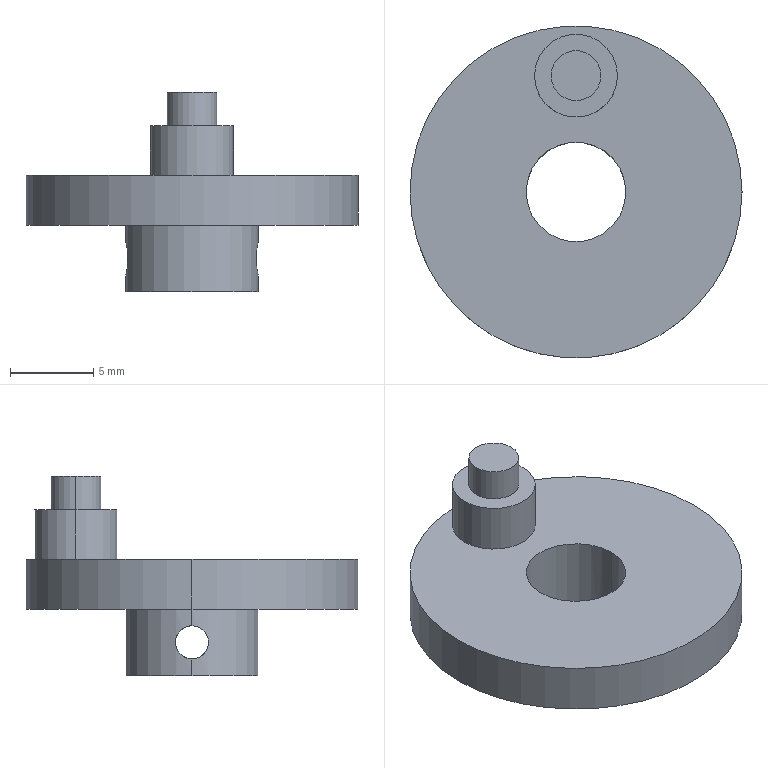Part | SolidWorks | features ICE 5, Extrusion 1 | 1 solid | 19 faces | box 20 x 20 x 12 mm | volume 1012 mm3 | cylinder 14 | plane 5 | commonest cylinder face diameters 2 x4 3 x2 5 x2 6 x2 8 x2 20 x2
STEP:
#1=CARTESIAN_POINT('',(3.,0.,-1.));
#2=VERTEX_POINT('',#1);
#3=CARTESIAN_POINT('',(3.,0.,-3.));
#4=VERTEX_POINT('',#3);
#5=CARTESIAN_POINT('',(3.,0.,-1.));
#6=CARTESIAN_POINT('',(3.,-0.1312,-1.));
#7=CARTESIAN_POINT('',(2.991,-0.2636,-1.027));
#8=CARTESIAN_POINT('',(2.96,-0.5049,-1.127));
#9=CARTESIAN_POINT('',(2.938,-0.6149,-1.201));
#10=CARTESIAN_POINT('',(2.893,-0.7996,-1.385));
#11=CARTESIAN_POINT('',(2.871,-0.8728,-1.494));
#12=CARTESIAN_POINT('',(2.838,-0.9739,-1.737));
#13=CARTESIAN_POINT('',(2.828,-1.,-1.868));
#14=CARTESIAN_POINT('',(2.828,-1.,-2.132));
#15=CARTESIAN_POINT('',(2.838,-0.9733,-2.264));
#16=CARTESIAN_POINT('',(2.871,-0.8731,-2.505));
#17=CARTESIAN_POINT('',(2.893,-0.7989,-2.615));
#18=CARTESIAN_POINT('',(2.938,-0.6156,-2.799));
#19=CARTESIAN_POINT('',(2.96,-0.5055,-2.873));
#20=CARTESIAN_POINT('',(2.991,-0.2638,-2.973));
#21=CARTESIAN_POINT('',(3.,-0.1331,-3.));
#22=CARTESIAN_POINT('',(3.,0.,-3.));
#23=B_SPLINE_CURVE_WITH_KNOTS('',3,(#5,#6,#7,#8,#9,#10,#11,#12,#13,#14,#15,#16,#17,#18,#19,#20,#21,#22),.UNSPECIFIED.,.F.,.F.,(4,2,2,2,2,2,2,2,4),(0.003149,0.003543,0.003936,0.00433,0.004723,0.005117,0.00551,0.005904,0.006298),.UNSPECIFIED.);
#24=EDGE_CURVE('',#2,#4,#23,.T.);
#25=ORIENTED_EDGE('',*,*,#24,.F.);
#26=CARTESIAN_POINT('',(4.,0.,-1.));
#27=VERTEX_POINT('',#26);
#28=CARTESIAN_POINT('',(-5.,0.,-1.));
#29=DIRECTION('',(1.,0.,0.));
#30=VECTOR('',#29,1000.);
#31=LINE('',#28,#30);
#32=EDGE_CURVE('',#2,#27,#31,.T.);
#33=ORIENTED_EDGE('',*,*,#32,.T.);
#34=CARTESIAN_POINT('',(4.,0.,-3.));
#35=VERTEX_POINT('',#34);
#36=CARTESIAN_POINT('',(4.,0.,-3.));
#37=CARTESIAN_POINT('',(4.,-0.1327,-3.));
#38=CARTESIAN_POINT('',(3.993,-0.2629,-2.974));
#39=CARTESIAN_POINT('',(3.97,-0.5049,-2.873));
#40=CARTESIAN_POINT('',(3.953,-0.6155,-2.799));
#41=CARTESIAN_POINT('',(3.92,-0.7991,-2.615));
#42=CARTESIAN_POINT('',(3.904,-0.8735,-2.504));
#43=CARTESIAN_POINT('',(3.88,-0.9734,-2.263));
#44=CARTESIAN_POINT('',(3.873,-0.9999,-2.131));
#45=CARTESIAN_POINT('',(3.873,-1.,-1.869));
#46=CARTESIAN_POINT('',(3.88,-0.974,-1.738));
#47=CARTESIAN_POINT('',(3.904,-0.8732,-1.495));
#48=CARTESIAN_POINT('',(3.92,-0.7996,-1.385));
#49=CARTESIAN_POINT('',(3.954,-0.6143,-1.2));
#50=CARTESIAN_POINT('',(3.97,-0.5041,-1.127));
#51=CARTESIAN_POINT('',(3.993,-0.2626,-1.026));
#52=CARTESIAN_POINT('',(4.,-0.1308,-1.));
#53=CARTESIAN_POINT('',(4.,0.,-1.));
#54=B_SPLINE_CURVE_WITH_KNOTS('',3,(#36,#37,#38,#39,#40,#41,#42,#43,#44,#45,#46,#47,#48,#49,#50,#51,#52,#53),.UNSPECIFIED.,.F.,.F.,(4,2,2,2,2,2,2,2,4),(0.,0.0003924,0.0007847,0.001177,0.001569,0.001962,0.002354,0.002747,0.003139),.UNSPECIFIED.);
#55=EDGE_CURVE('',#35,#27,#54,.T.);
#56=ORIENTED_EDGE('',*,*,#55,.F.);
#57=CARTESIAN_POINT('',(-5.,0.,-3.));
#58=DIRECTION('',(1.,0.,0.));
#59=VECTOR('',#58,1000.);
#60=LINE('',#57,#59);
#61=EDGE_CURVE('',#4,#35,#60,.T.);
#62=ORIENTED_EDGE('',*,*,#61,.F.);
#63=EDGE_LOOP('',(#25,#33,#56,#62));
#64=FACE_OUTER_BOUND('',#63,.T.);
#65=CARTESIAN_POINT('',(-5.,0.,-2.));
#66=DIRECTION('',(1.,0.,0.));
#67=DIRECTION('',(0.,0.,-1.));
#68=AXIS2_PLACEMENT_3D('',#65,#66,#67);
#69=CYLINDRICAL_SURFACE('',#68,1.);
#70=ADVANCED_FACE('',(#64),#69,.F.);
#71=CARTESIAN_POINT('',(-4.,0.,-1.));
#72=VERTEX_POINT('',#71);
#73=CARTESIAN_POINT('',(-4.,0.,-3.));
#74=VERTEX_POINT('',#73);
#75=CARTESIAN_POINT('',(-4.,0.,-1.));
#76=CARTESIAN_POINT('',(-4.,-0.1308,-1.));
#77=CARTESIAN_POINT('',(-3.993,-0.2629,-1.026));
#78=CARTESIAN_POINT('',(-3.97,-0.5038,-1.126));
#79=CARTESIAN_POINT('',(-3.954,-0.6146,-1.2));
#80=CARTESIAN_POINT('',(-3.92,-0.7991,-1.385));
#81=CARTESIAN_POINT('',(-3.904,-0.8727,-1.494));
#82=CARTESIAN_POINT('',(-3.88,-0.9739,-1.738));
#83=CARTESIAN_POINT('',(-3.873,-1.,-1.868));
#84=CARTESIAN_POINT('',(-3.873,-1.,-2.132));
#85=CARTESIAN_POINT('',(-3.88,-0.9737,-2.263));
#86=CARTESIAN_POINT('',(-3.904,-0.8736,-2.504));
#87=CARTESIAN_POINT('',(-3.92,-0.7992,-2.615));
#88=CARTESIAN_POINT('',(-3.953,-0.6158,-2.799));
#89=CARTESIAN_POINT('',(-3.97,-0.5048,-2.873));
#90=CARTESIAN_POINT('',(-3.993,-0.2641,-2.973));
#91=CARTESIAN_POINT('',(-4.,-0.1327,-3.));
#92=CARTESIAN_POINT('',(-4.,0.,-3.));
#93=B_SPLINE_CURVE_WITH_KNOTS('',3,(#75,#76,#77,#78,#79,#80,#81,#82,#83,#84,#85,#86,#87,#88,#89,#90,#91,#92),.UNSPECIFIED.,.F.,.F.,(4,2,2,2,2,2,2,2,4),(0.003139,0.003531,0.003923,0.004316,0.004708,0.0051,0.005493,0.005885,0.006277),.UNSPECIFIED.);
#94=EDGE_CURVE('',#72,#74,#93,.T.);
#95=ORIENTED_EDGE('',*,*,#94,.F.);
#96=CARTESIAN_POINT('',(-3.,0.,-1.));
#97=VERTEX_POINT('',#96);
#98=CARTESIAN_POINT('',(-5.,0.,-1.));
#99=DIRECTION('',(1.,0.,0.));
#100=VECTOR('',#99,1000.);
#101=LINE('',#98,#100);
#102=EDGE_CURVE('',#72,#97,#101,.T.);
#103=ORIENTED_EDGE('',*,*,#102,.T.);
#104=CARTESIAN_POINT('',(-3.,0.,-3.));
#105=VERTEX_POINT('',#104);
#106=CARTESIAN_POINT('',(-3.,0.,-3.));
#107=CARTESIAN_POINT('',(-3.,-0.1312,-3.));
#108=CARTESIAN_POINT('',(-2.991,-0.2636,-2.973));
#109=CARTESIAN_POINT('',(-2.96,-0.5049,-2.873));
#110=CARTESIAN_POINT('',(-2.938,-0.6149,-2.799));
#111=CARTESIAN_POINT('',(-2.893,-0.7996,-2.615));
#112=CARTESIAN_POINT('',(-2.871,-0.8728,-2.506));
#113=CARTESIAN_POINT('',(-2.838,-0.9739,-2.263));
#114=CARTESIAN_POINT('',(-2.828,-1.,-2.132));
#115=CARTESIAN_POINT('',(-2.828,-1.,-1.868));
#116=CARTESIAN_POINT('',(-2.838,-0.9733,-1.736));
#117=CARTESIAN_POINT('',(-2.871,-0.8731,-1.495));
#118=CARTESIAN_POINT('',(-2.893,-0.7989,-1.385));
#119=CARTESIAN_POINT('',(-2.938,-0.6156,-1.201));
#120=CARTESIAN_POINT('',(-2.96,-0.5055,-1.127));
#121=CARTESIAN_POINT('',(-2.991,-0.2638,-1.027));
#122=CARTESIAN_POINT('',(-3.,-0.1331,-1.));
#123=CARTESIAN_POINT('',(-3.,0.,-1.));
#124=B_SPLINE_CURVE_WITH_KNOTS('',3,(#106,#107,#108,#109,#110,#111,#112,#113,#114,#115,#116,#117,#118,#119,#120,#121,#122,#123),.UNSPECIFIED.,.F.,.F.,(4,2,2,2,2,2,2,2,4),(0.003149,0.003543,0.003936,0.00433,0.004723,0.005117,0.00551,0.005904,0.006298),.UNSPECIFIED.);
#125=EDGE_CURVE('',#105,#97,#124,.T.);
#126=ORIENTED_EDGE('',*,*,#125,.F.);
#127=CARTESIAN_POINT('',(-5.,0.,-3.));
#128=DIRECTION('',(1.,0.,0.));
#129=VECTOR('',#128,1000.);
#130=LINE('',#127,#129);
#131=EDGE_CURVE('',#74,#105,#130,.T.);
#132=ORIENTED_EDGE('',*,*,#131,.F.);
#133=EDGE_LOOP('',(#95,#103,#126,#132));
#134=FACE_OUTER_BOUND('',#133,.T.);
#135=CARTESIAN_POINT('',(-5.,0.,-2.));
#136=DIRECTION('',(1.,0.,0.));
#137=DIRECTION('',(0.,0.,-1.));
#138=AXIS2_PLACEMENT_3D('',#135,#136,#137);
#139=CYLINDRICAL_SURFACE('',#138,1.);
#140=ADVANCED_FACE('',(#134),#139,.F.);
#141=CARTESIAN_POINT('',(-4.,0.,-4.));
#142=VERTEX_POINT('',#141);
#143=CARTESIAN_POINT('',(4.,0.,-4.));
#144=VERTEX_POINT('',#143);
#145=CARTESIAN_POINT('',(0.,0.,-4.));
#146=DIRECTION('',(0.,0.,-1.));
#147=DIRECTION('',(-1.,0.,0.));
#148=AXIS2_PLACEMENT_3D('',#145,#146,#147);
#149=CIRCLE('',#148,4.);
#150=EDGE_CURVE('',#142,#144,#149,.T.);
#151=ORIENTED_EDGE('',*,*,#150,.F.);
#152=CARTESIAN_POINT('',(-4.,0.,-4.));
#153=DIRECTION('',(0.,0.,1.));
#154=VECTOR('',#153,1000.);
#155=LINE('',#152,#154);
#156=EDGE_CURVE('',#142,#74,#155,.T.);
#157=ORIENTED_EDGE('',*,*,#156,.T.);
#158=CARTESIAN_POINT('',(-4.,0.,-3.));
#159=CARTESIAN_POINT('',(-4.,0.1327,-3.));
#160=CARTESIAN_POINT('',(-3.993,0.2629,-2.974));
#161=CARTESIAN_POINT('',(-3.97,0.5049,-2.873));
#162=CARTESIAN_POINT('',(-3.953,0.6155,-2.799));
#163=CARTESIAN_POINT('',(-3.92,0.7991,-2.615));
#164=CARTESIAN_POINT('',(-3.904,0.8735,-2.504));
#165=CARTESIAN_POINT('',(-3.88,0.9734,-2.263));
#166=CARTESIAN_POINT('',(-3.873,0.9999,-2.131));
#167=CARTESIAN_POINT('',(-3.873,1.,-1.869));
#168=CARTESIAN_POINT('',(-3.88,0.974,-1.738));
#169=CARTESIAN_POINT('',(-3.904,0.8732,-1.495));
#170=CARTESIAN_POINT('',(-3.92,0.7996,-1.385));
#171=CARTESIAN_POINT('',(-3.954,0.6143,-1.2));
#172=CARTESIAN_POINT('',(-3.97,0.5041,-1.127));
#173=CARTESIAN_POINT('',(-3.993,0.2626,-1.026));
#174=CARTESIAN_POINT('',(-4.,0.1308,-1.));
#175=CARTESIAN_POINT('',(-4.,0.,-1.));
#176=B_SPLINE_CURVE_WITH_KNOTS('',3,(#158,#159,#160,#161,#162,#163,#164,#165,#166,#167,#168,#169,#170,#171,#172,#173,#174,#175),.UNSPECIFIED.,.F.,.F.,(4,2,2,2,2,2,2,2,4),(0.,0.0003924,0.0007847,0.001177,0.001569,0.001962,0.002354,0.002747,0.003139),.UNSPECIFIED.);
#177=EDGE_CURVE('',#74,#72,#176,.T.);
#178=ORIENTED_EDGE('',*,*,#177,.T.);
#179=CARTESIAN_POINT('',(-4.,0.,0.));
#180=VERTEX_POINT('',#179);
#181=CARTESIAN_POINT('',(-4.,0.,-4.));
#182=DIRECTION('',(0.,0.,1.));
#183=VECTOR('',#182,1000.);
#184=LINE('',#181,#183);
#185=EDGE_CURVE('',#72,#180,#184,.T.);
#186=ORIENTED_EDGE('',*,*,#185,.T.);
#187=CARTESIAN_POINT('',(4.,0.,0.));
#188=VERTEX_POINT('',#187);
#189=CARTESIAN_POINT('',(0.,0.,0.));
#190=DIRECTION('',(0.,0.,-1.));
#191=DIRECTION('',(1.,0.,0.));
#192=AXIS2_PLACEMENT_3D('',#189,#190,#191);
#193=CIRCLE('',#192,4.);
#194=EDGE_CURVE('',#180,#188,#193,.T.);
#195=ORIENTED_EDGE('',*,*,#194,.T.);
#196=CARTESIAN_POINT('',(4.,0.,-4.));
#197=DIRECTION('',(0.,0.,1.));
#198=VECTOR('',#197,1000.);
#199=LINE('',#196,#198);
#200=EDGE_CURVE('',#27,#188,#199,.T.);
#201=ORIENTED_EDGE('',*,*,#200,.F.);
#202=CARTESIAN_POINT('',(4.,0.,-1.));
#203=CARTESIAN_POINT('',(4.,0.1308,-1.));
#204=CARTESIAN_POINT('',(3.993,0.2629,-1.026));
#205=CARTESIAN_POINT('',(3.97,0.5038,-1.126));
#206=CARTESIAN_POINT('',(3.954,0.6146,-1.2));
#207=CARTESIAN_POINT('',(3.92,0.7991,-1.385));
#208=CARTESIAN_POINT('',(3.904,0.8727,-1.494));
#209=CARTESIAN_POINT('',(3.88,0.9739,-1.738));
#210=CARTESIAN_POINT('',(3.873,1.,-1.868));
#211=CARTESIAN_POINT('',(3.873,1.,-2.132));
#212=CARTESIAN_POINT('',(3.88,0.9737,-2.263));
#213=CARTESIAN_POINT('',(3.904,0.8736,-2.504));
#214=CARTESIAN_POINT('',(3.92,0.7992,-2.615));
#215=CARTESIAN_POINT('',(3.953,0.6158,-2.799));
#216=CARTESIAN_POINT('',(3.97,0.5048,-2.873));
#217=CARTESIAN_POINT('',(3.993,0.2641,-2.973));
#218=CARTESIAN_POINT('',(4.,0.1327,-3.));
#219=CARTESIAN_POINT('',(4.,0.,-3.));
#220=B_SPLINE_CURVE_WITH_KNOTS('',3,(#202,#203,#204,#205,#206,#207,#208,#209,#210,#211,#212,#213,#214,#215,#216,#217,#218,#219),.UNSPECIFIED.,.F.,.F.,(4,2,2,2,2,2,2,2,4),(0.003139,0.003531,0.003923,0.004316,0.004708,0.0051,0.005493,0.005885,0.006277),.UNSPECIFIED.);
#221=EDGE_CURVE('',#27,#35,#220,.T.);
#222=ORIENTED_EDGE('',*,*,#221,.T.);
#223=CARTESIAN_POINT('',(4.,0.,-4.));
#224=DIRECTION('',(0.,0.,1.));
#225=VECTOR('',#224,1000.);
#226=LINE('',#223,#225);
#227=EDGE_CURVE('',#144,#35,#226,.T.);
#228=ORIENTED_EDGE('',*,*,#227,.F.);
#229=EDGE_LOOP('',(#151,#157,#178,#186,#195,#201,#222,#228));
#230=FACE_OUTER_BOUND('',#229,.T.);
#231=CARTESIAN_POINT('',(0.,0.,-4.));
#232=DIRECTION('',(0.,0.,1.));
#233=DIRECTION('',(1.,0.,0.));
#234=AXIS2_PLACEMENT_3D('',#231,#232,#233);
#235=CYLINDRICAL_SURFACE('',#234,4.);
#236=ADVANCED_FACE('',(#230),#235,.T.);
#237=CARTESIAN_POINT('',(-3.,0.,3.));
#238=VERTEX_POINT('',#237);
#239=CARTESIAN_POINT('',(3.,0.,3.));
#240=VERTEX_POINT('',#239);
#241=CARTESIAN_POINT('',(0.,0.,3.));
#242=DIRECTION('',(0.,0.,1.));
#243=DIRECTION('',(1.,0.,0.));
#244=AXIS2_PLACEMENT_3D('',#241,#242,#243);
#245=CIRCLE('',#244,3.);
#246=EDGE_CURVE('',#238,#240,#245,.T.);
#247=ORIENTED_EDGE('',*,*,#246,.T.);
#248=CARTESIAN_POINT('',(3.,0.,24.));
#249=DIRECTION('',(0.,0.,-1.));
#250=VECTOR('',#249,1000.);
#251=LINE('',#248,#250);
#252=EDGE_CURVE('',#240,#2,#251,.T.);
#253=ORIENTED_EDGE('',*,*,#252,.T.);
#254=ORIENTED_EDGE('',*,*,#24,.T.);
#255=CARTESIAN_POINT('',(3.,0.,-4.));
#256=VERTEX_POINT('',#255);
#257=CARTESIAN_POINT('',(3.,0.,24.));
#258=DIRECTION('',(0.,0.,-1.));
#259=VECTOR('',#258,1000.);
#260=LINE('',#257,#259);
#261=EDGE_CURVE('',#4,#256,#260,.T.);
#262=ORIENTED_EDGE('',*,*,#261,.T.);
#263=CARTESIAN_POINT('',(-3.,0.,-4.));
#264=VERTEX_POINT('',#263);
#265=CARTESIAN_POINT('',(0.,0.,-4.));
#266=DIRECTION('',(0.,0.,-1.));
#267=DIRECTION('',(-1.,0.,0.));
#268=AXIS2_PLACEMENT_3D('',#265,#266,#267);
#269=CIRCLE('',#268,3.);
#270=EDGE_CURVE('',#256,#264,#269,.T.);
#271=ORIENTED_EDGE('',*,*,#270,.T.);
#272=CARTESIAN_POINT('',(-3.,0.,24.));
#273=DIRECTION('',(0.,0.,-1.));
#274=VECTOR('',#273,1000.);
#275=LINE('',#272,#274);
#276=EDGE_CURVE('',#105,#264,#275,.T.);
#277=ORIENTED_EDGE('',*,*,#276,.F.);
#278=ORIENTED_EDGE('',*,*,#125,.T.);
#279=CARTESIAN_POINT('',(-3.,0.,24.));
#280=DIRECTION('',(0.,0.,-1.));
#281=VECTOR('',#280,1000.);
#282=LINE('',#279,#281);
#283=EDGE_CURVE('',#238,#97,#282,.T.);
#284=ORIENTED_EDGE('',*,*,#283,.F.);
#285=EDGE_LOOP('',(#247,#253,#254,#262,#271,#277,#278,#284));
#286=FACE_OUTER_BOUND('',#285,.T.);
#287=CARTESIAN_POINT('',(0.,0.,24.));
#288=DIRECTION('',(0.,0.,-1.));
#289=DIRECTION('',(-1.,0.,0.));
#290=AXIS2_PLACEMENT_3D('',#287,#288,#289);
#291=CYLINDRICAL_SURFACE('',#290,3.);
#292=ADVANCED_FACE('',(#286),#291,.F.);
#293=CARTESIAN_POINT('',(1.5,7.,8.));
#294=VERTEX_POINT('',#293);
#295=CARTESIAN_POINT('',(-1.5,7.,8.));
#296=VERTEX_POINT('',#295);
#297=CARTESIAN_POINT('',(0.,7.,8.));
#298=DIRECTION('',(0.,0.,1.));
#299=DIRECTION('',(1.,0.,0.));
#300=AXIS2_PLACEMENT_3D('',#297,#298,#299);
#301=CIRCLE('',#300,1.5);
#302=EDGE_CURVE('',#294,#296,#301,.T.);
#303=ORIENTED_EDGE('',*,*,#302,.F.);
#304=CARTESIAN_POINT('',(1.5,7.,6.));
#305=VERTEX_POINT('',#304);
#306=CARTESIAN_POINT('',(1.5,7.,8.));
#307=DIRECTION('',(0.,0.,-1.));
#308=VECTOR('',#307,1000.);
#309=LINE('',#306,#308);
#310=EDGE_CURVE('',#294,#305,#309,.T.);
#311=ORIENTED_EDGE('',*,*,#310,.T.);
#312=CARTESIAN_POINT('',(-1.5,7.,6.));
#313=VERTEX_POINT('',#312);
#314=CARTESIAN_POINT('',(0.,7.,6.));
#315=DIRECTION('',(0.,0.,1.));
#316=DIRECTION('',(1.,0.,0.));
#317=AXIS2_PLACEMENT_3D('',#314,#315,#316);
#318=CIRCLE('',#317,1.5);
#319=EDGE_CURVE('',#305,#313,#318,.T.);
#320=ORIENTED_EDGE('',*,*,#319,.T.);
#321=CARTESIAN_POINT('',(-1.5,7.,8.));
#322=DIRECTION('',(0.,0.,-1.));
#323=VECTOR('',#322,1000.);
#324=LINE('',#321,#323);
#325=EDGE_CURVE('',#296,#313,#324,.T.);
#326=ORIENTED_EDGE('',*,*,#325,.F.);
#327=EDGE_LOOP('',(#303,#311,#320,#326));
#328=FACE_OUTER_BOUND('',#327,.T.);
#329=CARTESIAN_POINT('',(0.,7.,8.));
#330=DIRECTION('',(0.,0.,-1.));
#331=DIRECTION('',(-1.,0.,0.));
#332=AXIS2_PLACEMENT_3D('',#329,#330,#331);
#333=CYLINDRICAL_SURFACE('',#332,1.5);
#334=ADVANCED_FACE('',(#328),#333,.T.);
#335=CARTESIAN_POINT('',(2.5,7.,6.));
#336=VERTEX_POINT('',#335);
#337=CARTESIAN_POINT('',(-2.5,7.,6.));
#338=VERTEX_POINT('',#337);
#339=CARTESIAN_POINT('',(0.,7.,6.));
#340=DIRECTION('',(0.,0.,1.));
#341=DIRECTION('',(1.,0.,0.));
#342=AXIS2_PLACEMENT_3D('',#339,#340,#341);
#343=CIRCLE('',#342,2.5);
#344=EDGE_CURVE('',#336,#338,#343,.T.);
#345=ORIENTED_EDGE('',*,*,#344,.F.);
#346=CARTESIAN_POINT('',(2.5,7.,3.));
#347=VERTEX_POINT('',#346);
#348=CARTESIAN_POINT('',(2.5,7.,6.));
#349=DIRECTION('',(0.,0.,-1.));
#350=VECTOR('',#349,1000.);
#351=LINE('',#348,#350);
#352=EDGE_CURVE('',#336,#347,#351,.T.);
#353=ORIENTED_EDGE('',*,*,#352,.T.);
#354=CARTESIAN_POINT('',(-2.5,7.,3.));
#355=VERTEX_POINT('',#354);
#356=CARTESIAN_POINT('',(0.,7.,3.));
#357=DIRECTION('',(0.,0.,1.));
#358=DIRECTION('',(1.,0.,0.));
#359=AXIS2_PLACEMENT_3D('',#356,#357,#358);
#360=CIRCLE('',#359,2.5);
#361=EDGE_CURVE('',#347,#355,#360,.T.);
#362=ORIENTED_EDGE('',*,*,#361,.T.);
#363=CARTESIAN_POINT('',(-2.5,7.,6.));
#364=DIRECTION('',(0.,0.,-1.));
#365=VECTOR('',#364,1000.);
#366=LINE('',#363,#365);
#367=EDGE_CURVE('',#338,#355,#366,.T.);
#368=ORIENTED_EDGE('',*,*,#367,.F.);
#369=EDGE_LOOP('',(#345,#353,#362,#368));
#370=FACE_OUTER_BOUND('',#369,.T.);
#371=CARTESIAN_POINT('',(0.,7.,6.));
#372=DIRECTION('',(0.,0.,-1.));
#373=DIRECTION('',(-1.,0.,0.));
#374=AXIS2_PLACEMENT_3D('',#371,#372,#373);
#375=CYLINDRICAL_SURFACE('',#374,2.5);
#376=ADVANCED_FACE('',(#370),#375,.T.);
#377=CARTESIAN_POINT('',(10.,0.,3.));
#378=VERTEX_POINT('',#377);
#379=CARTESIAN_POINT('',(-10.,0.,3.));
#380=VERTEX_POINT('',#379);
#381=CARTESIAN_POINT('',(0.,0.,3.));
#382=DIRECTION('',(0.,0.,1.));
#383=DIRECTION('',(1.,0.,0.));
#384=AXIS2_PLACEMENT_3D('',#381,#382,#383);
#385=CIRCLE('',#384,10.);
#386=EDGE_CURVE('',#378,#380,#385,.T.);
#387=ORIENTED_EDGE('',*,*,#386,.F.);
#388=CARTESIAN_POINT('',(10.,0.,0.));
#389=VERTEX_POINT('',#388);
#390=CARTESIAN_POINT('',(10.,0.,3.));
#391=DIRECTION('',(0.,0.,-1.));
#392=VECTOR('',#391,1000.);
#393=LINE('',#390,#392);
#394=EDGE_CURVE('',#378,#389,#393,.T.);
#395=ORIENTED_EDGE('',*,*,#394,.T.);
#396=CARTESIAN_POINT('',(-10.,0.,0.));
#397=VERTEX_POINT('',#396);
#398=CARTESIAN_POINT('',(0.,0.,0.));
#399=DIRECTION('',(0.,0.,1.));
#400=DIRECTION('',(1.,0.,0.));
#401=AXIS2_PLACEMENT_3D('',#398,#399,#400);
#402=CIRCLE('',#401,10.);
#403=EDGE_CURVE('',#389,#397,#402,.T.);
#404=ORIENTED_EDGE('',*,*,#403,.T.);
#405=CARTESIAN_POINT('',(-10.,0.,3.));
#406=DIRECTION('',(0.,0.,-1.));
#407=VECTOR('',#406,1000.);
#408=LINE('',#405,#407);
#409=EDGE_CURVE('',#380,#397,#408,.T.);
#410=ORIENTED_EDGE('',*,*,#409,.F.);
#411=EDGE_LOOP('',(#387,#395,#404,#410));
#412=FACE_OUTER_BOUND('',#411,.T.);
#413=CARTESIAN_POINT('',(0.,0.,3.));
#414=DIRECTION('',(0.,0.,-1.));
#415=DIRECTION('',(-1.,0.,0.));
#416=AXIS2_PLACEMENT_3D('',#413,#414,#415);
#417=CYLINDRICAL_SURFACE('',#416,10.);
#418=ADVANCED_FACE('',(#412),#417,.T.);
#419=CARTESIAN_POINT('',(0.,0.,0.));
#420=DIRECTION('',(0.,0.,1.));
#421=DIRECTION('',(1.,0.,0.));
#422=AXIS2_PLACEMENT_3D('',#419,#420,#421);
#423=CIRCLE('',#422,10.);
#424=EDGE_CURVE('',#397,#389,#423,.T.);
#425=ORIENTED_EDGE('',*,*,#424,.F.);
#426=ORIENTED_EDGE('',*,*,#403,.F.);
#427=EDGE_LOOP('',(#425,#426));
#428=FACE_OUTER_BOUND('',#427,.T.);
#429=CARTESIAN_POINT('',(0.,0.,0.));
#430=DIRECTION('',(0.,0.,-1.));
#431=DIRECTION('',(1.,0.,0.));
#432=AXIS2_PLACEMENT_3D('',#429,#430,#431);
#433=CIRCLE('',#432,4.);
#434=EDGE_CURVE('',#188,#180,#433,.T.);
#435=ORIENTED_EDGE('',*,*,#434,.F.);
#436=ORIENTED_EDGE('',*,*,#194,.F.);
#437=EDGE_LOOP('',(#435,#436));
#438=FACE_BOUND('',#437,.T.);
#439=CARTESIAN_POINT('',(0.,0.,0.));
#440=DIRECTION('',(0.,0.,1.));
#441=DIRECTION('',(1.,0.,0.));
#442=AXIS2_PLACEMENT_3D('',#439,#440,#441);
#443=PLANE('',#442);
#444=ADVANCED_FACE('',(#428,#438),#443,.F.);
#445=CARTESIAN_POINT('',(0.,7.,6.));
#446=DIRECTION('',(0.,0.,1.));
#447=DIRECTION('',(1.,0.,0.));
#448=AXIS2_PLACEMENT_3D('',#445,#446,#447);
#449=CIRCLE('',#448,2.5);
#450=EDGE_CURVE('',#338,#336,#449,.T.);
#451=ORIENTED_EDGE('',*,*,#450,.T.);
#452=ORIENTED_EDGE('',*,*,#344,.T.);
#453=EDGE_LOOP('',(#451,#452));
#454=FACE_OUTER_BOUND('',#453,.T.);
#455=CARTESIAN_POINT('',(0.,7.,6.));
#456=DIRECTION('',(0.,0.,1.));
#457=DIRECTION('',(1.,0.,0.));
#458=AXIS2_PLACEMENT_3D('',#455,#456,#457);
#459=CIRCLE('',#458,1.5);
#460=EDGE_CURVE('',#313,#305,#459,.T.);
#461=ORIENTED_EDGE('',*,*,#460,.F.);
#462=ORIENTED_EDGE('',*,*,#319,.F.);
#463=EDGE_LOOP('',(#461,#462));
#464=FACE_BOUND('',#463,.T.);
#465=CARTESIAN_POINT('',(0.,7.,6.));
#466=DIRECTION('',(0.,0.,1.));
#467=DIRECTION('',(1.,0.,0.));
#468=AXIS2_PLACEMENT_3D('',#465,#466,#467);
#469=PLANE('',#468);
#470=ADVANCED_FACE('',(#454,#464),#469,.T.);
#471=ORIENTED_EDGE('',*,*,#246,.F.);
#472=CARTESIAN_POINT('',(0.,0.,3.));
#473=DIRECTION('',(0.,0.,1.));
#474=DIRECTION('',(1.,0.,0.));
#475=AXIS2_PLACEMENT_3D('',#472,#473,#474);
#476=CIRCLE('',#475,3.);
#477=EDGE_CURVE('',#240,#238,#476,.T.);
#478=ORIENTED_EDGE('',*,*,#477,.F.);
#479=EDGE_LOOP('',(#471,#478));
#480=FACE_BOUND('',#479,.T.);
#481=CARTESIAN_POINT('',(0.,0.,3.));
#482=DIRECTION('',(0.,0.,1.));
#483=DIRECTION('',(1.,0.,0.));
#484=AXIS2_PLACEMENT_3D('',#481,#482,#483);
#485=CIRCLE('',#484,10.);
#486=EDGE_CURVE('',#380,#378,#485,.T.);
#487=ORIENTED_EDGE('',*,*,#486,.T.);
#488=ORIENTED_EDGE('',*,*,#386,.T.);
#489=EDGE_LOOP('',(#487,#488));
#490=FACE_OUTER_BOUND('',#489,.T.);
#491=CARTESIAN_POINT('',(0.,7.,3.));
#492=DIRECTION('',(0.,0.,1.));
#493=DIRECTION('',(1.,0.,0.));
#494=AXIS2_PLACEMENT_3D('',#491,#492,#493);
#495=CIRCLE('',#494,2.5);
#496=EDGE_CURVE('',#355,#347,#495,.T.);
#497=ORIENTED_EDGE('',*,*,#496,.F.);
#498=ORIENTED_EDGE('',*,*,#361,.F.);
#499=EDGE_LOOP('',(#497,#498));
#500=FACE_BOUND('',#499,.T.);
#501=CARTESIAN_POINT('',(0.,0.,3.));
#502=DIRECTION('',(0.,0.,1.));
#503=DIRECTION('',(1.,0.,0.));
#504=AXIS2_PLACEMENT_3D('',#501,#502,#503);
#505=PLANE('',#504);
#506=ADVANCED_FACE('',(#480,#490,#500),#505,.T.);
#507=ORIENTED_EDGE('',*,*,#394,.F.);
#508=ORIENTED_EDGE('',*,*,#486,.F.);
#509=ORIENTED_EDGE('',*,*,#409,.T.);
#510=ORIENTED_EDGE('',*,*,#424,.T.);
#511=EDGE_LOOP('',(#507,#508,#509,#510));
#512=FACE_OUTER_BOUND('',#511,.T.);
#513=CARTESIAN_POINT('',(0.,0.,3.));
#514=DIRECTION('',(0.,0.,-1.));
#515=DIRECTION('',(-1.,0.,0.));
#516=AXIS2_PLACEMENT_3D('',#513,#514,#515);
#517=CYLINDRICAL_SURFACE('',#516,10.);
#518=ADVANCED_FACE('',(#512),#517,.T.);
#519=ORIENTED_EDGE('',*,*,#352,.F.);
#520=ORIENTED_EDGE('',*,*,#450,.F.);
#521=ORIENTED_EDGE('',*,*,#367,.T.);
#522=ORIENTED_EDGE('',*,*,#496,.T.);
#523=EDGE_LOOP('',(#519,#520,#521,#522));
#524=FACE_OUTER_BOUND('',#523,.T.);
#525=CARTESIAN_POINT('',(0.,7.,6.));
#526=DIRECTION('',(0.,0.,-1.));
#527=DIRECTION('',(-1.,0.,0.));
#528=AXIS2_PLACEMENT_3D('',#525,#526,#527);
#529=CYLINDRICAL_SURFACE('',#528,2.5);
#530=ADVANCED_FACE('',(#524),#529,.T.);
#531=ORIENTED_EDGE('',*,*,#310,.F.);
#532=CARTESIAN_POINT('',(0.,7.,8.));
#533=DIRECTION('',(0.,0.,1.));
#534=DIRECTION('',(1.,0.,0.));
#535=AXIS2_PLACEMENT_3D('',#532,#533,#534);
#536=CIRCLE('',#535,1.5);
#537=EDGE_CURVE('',#296,#294,#536,.T.);
#538=ORIENTED_EDGE('',*,*,#537,.F.);
#539=ORIENTED_EDGE('',*,*,#325,.T.);
#540=ORIENTED_EDGE('',*,*,#460,.T.);
#541=EDGE_LOOP('',(#531,#538,#539,#540));
#542=FACE_OUTER_BOUND('',#541,.T.);
#543=CARTESIAN_POINT('',(0.,7.,8.));
#544=DIRECTION('',(0.,0.,-1.));
#545=DIRECTION('',(-1.,0.,0.));
#546=AXIS2_PLACEMENT_3D('',#543,#544,#545);
#547=CYLINDRICAL_SURFACE('',#546,1.5);
#548=ADVANCED_FACE('',(#542),#547,.T.);
#549=ORIENTED_EDGE('',*,*,#537,.T.);
#550=ORIENTED_EDGE('',*,*,#302,.T.);
#551=EDGE_LOOP('',(#549,#550));
#552=FACE_OUTER_BOUND('',#551,.T.);
#553=CARTESIAN_POINT('',(0.,7.,8.));
#554=DIRECTION('',(0.,0.,1.));
#555=DIRECTION('',(1.,0.,0.));
#556=AXIS2_PLACEMENT_3D('',#553,#554,#555);
#557=PLANE('',#556);
#558=ADVANCED_FACE('',(#552),#557,.T.);
#559=ORIENTED_EDGE('',*,*,#252,.F.);
#560=ORIENTED_EDGE('',*,*,#477,.T.);
#561=ORIENTED_EDGE('',*,*,#283,.T.);
#562=CARTESIAN_POINT('',(-3.,0.,-1.));
#563=CARTESIAN_POINT('',(-3.,0.1332,-1.));
#564=CARTESIAN_POINT('',(-2.991,0.2638,-1.027));
#565=CARTESIAN_POINT('',(-2.96,0.5056,-1.127));
#566=CARTESIAN_POINT('',(-2.938,0.6159,-1.202));
#567=CARTESIAN_POINT('',(-2.893,0.7989,-1.385));
#568=CARTESIAN_POINT('',(-2.871,0.8732,-1.496));
#569=CARTESIAN_POINT('',(-2.838,0.9732,-1.736));
#570=CARTESIAN_POINT('',(-2.828,0.9999,-1.868));
#571=CARTESIAN_POINT('',(-2.828,1.,-2.131));
#572=CARTESIAN_POINT('',(-2.838,0.9739,-2.262));
#573=CARTESIAN_POINT('',(-2.871,0.8726,-2.506));
#574=CARTESIAN_POINT('',(-2.893,0.7989,-2.615));
#575=CARTESIAN_POINT('',(-2.938,0.6148,-2.799));
#576=CARTESIAN_POINT('',(-2.96,0.5044,-2.873));
#577=CARTESIAN_POINT('',(-2.991,0.2636,-2.973));
#578=CARTESIAN_POINT('',(-3.,0.1312,-3.));
#579=CARTESIAN_POINT('',(-3.,0.,-3.));
#580=B_SPLINE_CURVE_WITH_KNOTS('',3,(#562,#563,#564,#565,#566,#567,#568,#569,#570,#571,#572,#573,#574,#575,#576,#577,#578,#579),.UNSPECIFIED.,.F.,.F.,(4,2,2,2,2,2,2,2,4),(0.,0.0003936,0.0007873,0.001181,0.001575,0.001968,0.002362,0.002756,0.003149),.UNSPECIFIED.);
#581=EDGE_CURVE('',#97,#105,#580,.T.);
#582=ORIENTED_EDGE('',*,*,#581,.T.);
#583=ORIENTED_EDGE('',*,*,#276,.T.);
#584=CARTESIAN_POINT('',(0.,0.,-4.));
#585=DIRECTION('',(0.,0.,-1.));
#586=DIRECTION('',(-1.,0.,0.));
#587=AXIS2_PLACEMENT_3D('',#584,#585,#586);
#588=CIRCLE('',#587,3.);
#589=EDGE_CURVE('',#264,#256,#588,.T.);
#590=ORIENTED_EDGE('',*,*,#589,.T.);
#591=ORIENTED_EDGE('',*,*,#261,.F.);
#592=CARTESIAN_POINT('',(3.,0.,-3.));
#593=CARTESIAN_POINT('',(3.,0.1332,-3.));
#594=CARTESIAN_POINT('',(2.991,0.2638,-2.973));
#595=CARTESIAN_POINT('',(2.96,0.5056,-2.873));
#596=CARTESIAN_POINT('',(2.938,0.6159,-2.798));
#597=CARTESIAN_POINT('',(2.893,0.7989,-2.615));
#598=CARTESIAN_POINT('',(2.871,0.8732,-2.504));
#599=CARTESIAN_POINT('',(2.838,0.9732,-2.264));
#600=CARTESIAN_POINT('',(2.828,0.9999,-2.132));
#601=CARTESIAN_POINT('',(2.828,1.,-1.869));
#602=CARTESIAN_POINT('',(2.838,0.9739,-1.738));
#603=CARTESIAN_POINT('',(2.871,0.8726,-1.494));
#604=CARTESIAN_POINT('',(2.893,0.7989,-1.385));
#605=CARTESIAN_POINT('',(2.938,0.6148,-1.201));
#606=CARTESIAN_POINT('',(2.96,0.5044,-1.127));
#607=CARTESIAN_POINT('',(2.991,0.2636,-1.027));
#608=CARTESIAN_POINT('',(3.,0.1312,-1.));
#609=CARTESIAN_POINT('',(3.,0.,-1.));
#610=B_SPLINE_CURVE_WITH_KNOTS('',3,(#592,#593,#594,#595,#596,#597,#598,#599,#600,#601,#602,#603,#604,#605,#606,#607,#608,#609),.UNSPECIFIED.,.F.,.F.,(4,2,2,2,2,2,2,2,4),(0.,0.0003936,0.0007873,0.001181,0.001575,0.001968,0.002362,0.002756,0.003149),.UNSPECIFIED.);
#611=EDGE_CURVE('',#4,#2,#610,.T.);
#612=ORIENTED_EDGE('',*,*,#611,.T.);
#613=EDGE_LOOP('',(#559,#560,#561,#582,#583,#590,#591,#612));
#614=FACE_OUTER_BOUND('',#613,.T.);
#615=CARTESIAN_POINT('',(0.,0.,24.));
#616=DIRECTION('',(0.,0.,-1.));
#617=DIRECTION('',(-1.,0.,0.));
#618=AXIS2_PLACEMENT_3D('',#615,#616,#617);
#619=CYLINDRICAL_SURFACE('',#618,3.);
#620=ADVANCED_FACE('',(#614),#619,.F.);
#621=CARTESIAN_POINT('',(0.,0.,-4.));
#622=DIRECTION('',(0.,0.,-1.));
#623=DIRECTION('',(-1.,0.,0.));
#624=AXIS2_PLACEMENT_3D('',#621,#622,#623);
#625=CIRCLE('',#624,4.);
#626=EDGE_CURVE('',#144,#142,#625,.T.);
#627=ORIENTED_EDGE('',*,*,#626,.T.);
#628=ORIENTED_EDGE('',*,*,#150,.T.);
#629=EDGE_LOOP('',(#627,#628));
#630=FACE_OUTER_BOUND('',#629,.T.);
#631=ORIENTED_EDGE('',*,*,#589,.F.);
#632=ORIENTED_EDGE('',*,*,#270,.F.);
#633=EDGE_LOOP('',(#631,#632));
#634=FACE_BOUND('',#633,.T.);
#635=CARTESIAN_POINT('',(0.,0.,-4.));
#636=DIRECTION('',(0.,0.,-1.));
#637=DIRECTION('',(-1.,0.,0.));
#638=AXIS2_PLACEMENT_3D('',#635,#636,#637);
#639=PLANE('',#638);
#640=ADVANCED_FACE('',(#630,#634),#639,.T.);
#641=ORIENTED_EDGE('',*,*,#156,.F.);
#642=ORIENTED_EDGE('',*,*,#626,.F.);
#643=ORIENTED_EDGE('',*,*,#227,.T.);
#644=ORIENTED_EDGE('',*,*,#55,.T.);
#645=ORIENTED_EDGE('',*,*,#200,.T.);
#646=ORIENTED_EDGE('',*,*,#434,.T.);
#647=ORIENTED_EDGE('',*,*,#185,.F.);
#648=ORIENTED_EDGE('',*,*,#94,.T.);
#649=EDGE_LOOP('',(#641,#642,#643,#644,#645,#646,#647,#648));
#650=FACE_OUTER_BOUND('',#649,.T.);
#651=CARTESIAN_POINT('',(0.,0.,-4.));
#652=DIRECTION('',(0.,0.,1.));
#653=DIRECTION('',(1.,0.,0.));
#654=AXIS2_PLACEMENT_3D('',#651,#652,#653);
#655=CYLINDRICAL_SURFACE('',#654,4.);
#656=ADVANCED_FACE('',(#650),#655,.T.);
#657=ORIENTED_EDGE('',*,*,#102,.F.);
#658=ORIENTED_EDGE('',*,*,#177,.F.);
#659=ORIENTED_EDGE('',*,*,#131,.T.);
#660=ORIENTED_EDGE('',*,*,#581,.F.);
#661=EDGE_LOOP('',(#657,#658,#659,#660));
#662=FACE_OUTER_BOUND('',#661,.T.);
#663=CARTESIAN_POINT('',(-5.,0.,-2.));
#664=DIRECTION('',(1.,0.,0.));
#665=DIRECTION('',(0.,0.,-1.));
#666=AXIS2_PLACEMENT_3D('',#663,#664,#665);
#667=CYLINDRICAL_SURFACE('',#666,1.);
#668=ADVANCED_FACE('',(#662),#667,.F.);
#669=ORIENTED_EDGE('',*,*,#32,.F.);
#670=ORIENTED_EDGE('',*,*,#611,.F.);
#671=ORIENTED_EDGE('',*,*,#61,.T.);
#672=ORIENTED_EDGE('',*,*,#221,.F.);
#673=EDGE_LOOP('',(#669,#670,#671,#672));
#674=FACE_OUTER_BOUND('',#673,.T.);
#675=CARTESIAN_POINT('',(-5.,0.,-2.));
#676=DIRECTION('',(1.,0.,0.));
#677=DIRECTION('',(0.,0.,-1.));
#678=AXIS2_PLACEMENT_3D('',#675,#676,#677);
#679=CYLINDRICAL_SURFACE('',#678,1.);
#680=ADVANCED_FACE('',(#674),#679,.F.);
#681=CLOSED_SHELL('',(#70,#140,#236,#292,#334,#376,#418,#444,#470,#506,#518,#530,#548,#558,#620,#640,#656,#668,#680));
#682=MANIFOLD_SOLID_BREP('',#681);
#683=CARTESIAN_POINT('',(0.,0.,0.));
#684=DIRECTION('',(0.,0.,1.));
#685=DIRECTION('',(1.,0.,0.));
#686=AXIS2_PLACEMENT_3D('',#683,#684,#685);
#687=(LENGTH_UNIT()NAMED_UNIT(*)SI_UNIT(.MILLI.,.METRE.));
#688=UNCERTAINTY_MEASURE_WITH_UNIT(LENGTH_MEASURE(0.00001),#687,'','');
#689=(NAMED_UNIT(*)PLANE_ANGLE_UNIT()SI_UNIT($,.RADIAN.));
#690=(NAMED_UNIT(*)SI_UNIT($,.STERADIAN.)SOLID_ANGLE_UNIT());
#691=(GEOMETRIC_REPRESENTATION_CONTEXT(3)GLOBAL_UNCERTAINTY_ASSIGNED_CONTEXT((#688))GLOBAL_UNIT_ASSIGNED_CONTEXT((#687,#689,#690))REPRESENTATION_CONTEXT('',''));
#692=ADVANCED_BREP_SHAPE_REPRESENTATION('',(#682,#686),#691);